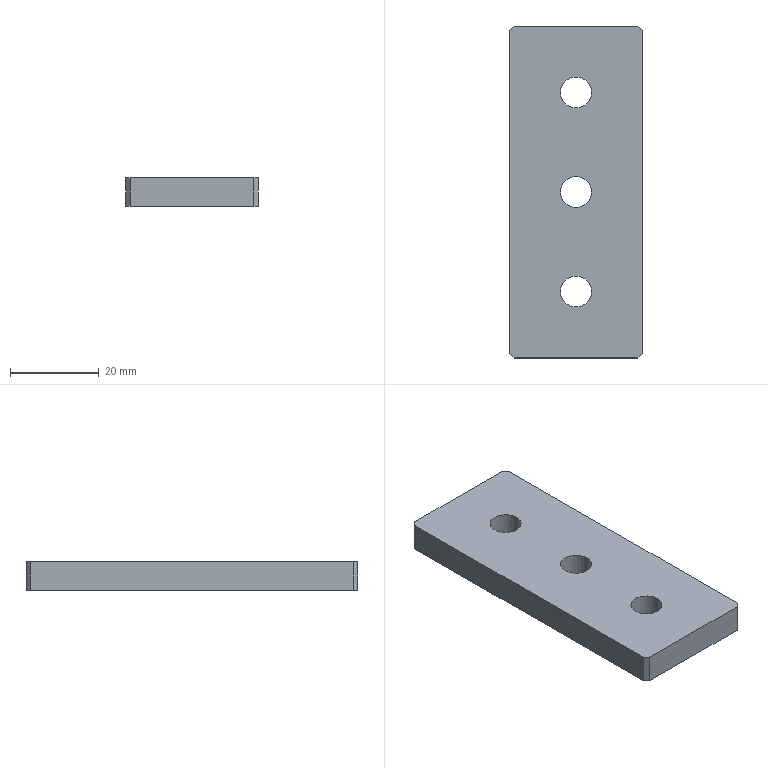Part | SolidWorks | features Chamfer 1, Extrusion 1, HoleWzd 1 | 1 solid | 16 faces | box 30 x 75 x 6.5 mm | volume 13862 mm3 | plane 10 | cylinder 6 | commonest cylinder face diameters 7 x6
STEP:
#1=CARTESIAN_POINT('',(-3.5,0.,0.));
#2=VERTEX_POINT('',#1);
#3=CARTESIAN_POINT('',(3.5,0.,0.));
#4=VERTEX_POINT('',#3);
#5=CARTESIAN_POINT('',(0.,0.,0.));
#6=DIRECTION('',(0.,0.,1.));
#7=DIRECTION('',(1.,0.,0.));
#8=AXIS2_PLACEMENT_3D('',#5,#6,#7);
#9=CIRCLE('',#8,3.5);
#10=EDGE_CURVE('',#2,#4,#9,.T.);
#11=ORIENTED_EDGE('',*,*,#10,.F.);
#12=CARTESIAN_POINT('',(-3.5,0.,6.5));
#13=VERTEX_POINT('',#12);
#14=CARTESIAN_POINT('',(-3.5,0.,6.5));
#15=DIRECTION('',(0.,0.,1.));
#16=VECTOR('',#15,1000.);
#17=LINE('',#14,#16);
#18=EDGE_CURVE('',#2,#13,#17,.T.);
#19=ORIENTED_EDGE('',*,*,#18,.T.);
#20=CARTESIAN_POINT('',(3.5,0.,6.5));
#21=VERTEX_POINT('',#20);
#22=CARTESIAN_POINT('',(0.,0.,6.5));
#23=DIRECTION('',(0.,0.,1.));
#24=DIRECTION('',(1.,0.,0.));
#25=AXIS2_PLACEMENT_3D('',#22,#23,#24);
#26=CIRCLE('',#25,3.5);
#27=EDGE_CURVE('',#13,#21,#26,.T.);
#28=ORIENTED_EDGE('',*,*,#27,.T.);
#29=CARTESIAN_POINT('',(3.5,0.,6.5));
#30=DIRECTION('',(0.,0.,1.));
#31=VECTOR('',#30,1000.);
#32=LINE('',#29,#31);
#33=EDGE_CURVE('',#4,#21,#32,.T.);
#34=ORIENTED_EDGE('',*,*,#33,.F.);
#35=EDGE_LOOP('',(#11,#19,#28,#34));
#36=FACE_OUTER_BOUND('',#35,.T.);
#37=CARTESIAN_POINT('',(0.,0.,6.5));
#38=DIRECTION('',(0.,0.,1.));
#39=DIRECTION('',(1.,0.,0.));
#40=AXIS2_PLACEMENT_3D('',#37,#38,#39);
#41=CYLINDRICAL_SURFACE('',#40,3.5);
#42=ADVANCED_FACE('',(#36),#41,.F.);
#43=CARTESIAN_POINT('',(-3.5,-22.5,0.));
#44=VERTEX_POINT('',#43);
#45=CARTESIAN_POINT('',(3.5,-22.5,0.));
#46=VERTEX_POINT('',#45);
#47=CARTESIAN_POINT('',(0.,-22.5,0.));
#48=DIRECTION('',(0.,0.,1.));
#49=DIRECTION('',(1.,0.,0.));
#50=AXIS2_PLACEMENT_3D('',#47,#48,#49);
#51=CIRCLE('',#50,3.5);
#52=EDGE_CURVE('',#44,#46,#51,.T.);
#53=ORIENTED_EDGE('',*,*,#52,.F.);
#54=CARTESIAN_POINT('',(-3.5,-22.5,6.5));
#55=VERTEX_POINT('',#54);
#56=CARTESIAN_POINT('',(-3.5,-22.5,6.5));
#57=DIRECTION('',(0.,0.,1.));
#58=VECTOR('',#57,1000.);
#59=LINE('',#56,#58);
#60=EDGE_CURVE('',#44,#55,#59,.T.);
#61=ORIENTED_EDGE('',*,*,#60,.T.);
#62=CARTESIAN_POINT('',(3.5,-22.5,6.5));
#63=VERTEX_POINT('',#62);
#64=CARTESIAN_POINT('',(0.,-22.5,6.5));
#65=DIRECTION('',(0.,0.,1.));
#66=DIRECTION('',(1.,0.,0.));
#67=AXIS2_PLACEMENT_3D('',#64,#65,#66);
#68=CIRCLE('',#67,3.5);
#69=EDGE_CURVE('',#55,#63,#68,.T.);
#70=ORIENTED_EDGE('',*,*,#69,.T.);
#71=CARTESIAN_POINT('',(3.5,-22.5,6.5));
#72=DIRECTION('',(0.,0.,1.));
#73=VECTOR('',#72,1000.);
#74=LINE('',#71,#73);
#75=EDGE_CURVE('',#46,#63,#74,.T.);
#76=ORIENTED_EDGE('',*,*,#75,.F.);
#77=EDGE_LOOP('',(#53,#61,#70,#76));
#78=FACE_OUTER_BOUND('',#77,.T.);
#79=CARTESIAN_POINT('',(0.,-22.5,6.5));
#80=DIRECTION('',(0.,0.,1.));
#81=DIRECTION('',(1.,0.,0.));
#82=AXIS2_PLACEMENT_3D('',#79,#80,#81);
#83=CYLINDRICAL_SURFACE('',#82,3.5);
#84=ADVANCED_FACE('',(#78),#83,.F.);
#85=CARTESIAN_POINT('',(-3.5,22.5,0.));
#86=VERTEX_POINT('',#85);
#87=CARTESIAN_POINT('',(3.5,22.5,0.));
#88=VERTEX_POINT('',#87);
#89=CARTESIAN_POINT('',(0.,22.5,0.));
#90=DIRECTION('',(0.,0.,1.));
#91=DIRECTION('',(1.,0.,0.));
#92=AXIS2_PLACEMENT_3D('',#89,#90,#91);
#93=CIRCLE('',#92,3.5);
#94=EDGE_CURVE('',#86,#88,#93,.T.);
#95=ORIENTED_EDGE('',*,*,#94,.F.);
#96=CARTESIAN_POINT('',(-3.5,22.5,6.5));
#97=VERTEX_POINT('',#96);
#98=CARTESIAN_POINT('',(-3.5,22.5,6.5));
#99=DIRECTION('',(0.,0.,1.));
#100=VECTOR('',#99,1000.);
#101=LINE('',#98,#100);
#102=EDGE_CURVE('',#86,#97,#101,.T.);
#103=ORIENTED_EDGE('',*,*,#102,.T.);
#104=CARTESIAN_POINT('',(3.5,22.5,6.5));
#105=VERTEX_POINT('',#104);
#106=CARTESIAN_POINT('',(0.,22.5,6.5));
#107=DIRECTION('',(0.,0.,1.));
#108=DIRECTION('',(1.,0.,0.));
#109=AXIS2_PLACEMENT_3D('',#106,#107,#108);
#110=CIRCLE('',#109,3.5);
#111=EDGE_CURVE('',#97,#105,#110,.T.);
#112=ORIENTED_EDGE('',*,*,#111,.T.);
#113=CARTESIAN_POINT('',(3.5,22.5,6.5));
#114=DIRECTION('',(0.,0.,1.));
#115=VECTOR('',#114,1000.);
#116=LINE('',#113,#115);
#117=EDGE_CURVE('',#88,#105,#116,.T.);
#118=ORIENTED_EDGE('',*,*,#117,.F.);
#119=EDGE_LOOP('',(#95,#103,#112,#118));
#120=FACE_OUTER_BOUND('',#119,.T.);
#121=CARTESIAN_POINT('',(0.,22.5,6.5));
#122=DIRECTION('',(0.,0.,1.));
#123=DIRECTION('',(1.,0.,0.));
#124=AXIS2_PLACEMENT_3D('',#121,#122,#123);
#125=CYLINDRICAL_SURFACE('',#124,3.5);
#126=ADVANCED_FACE('',(#120),#125,.F.);
#127=CARTESIAN_POINT('',(15.,-36.5,0.));
#128=VERTEX_POINT('',#127);
#129=CARTESIAN_POINT('',(15.,36.5,0.));
#130=VERTEX_POINT('',#129);
#131=CARTESIAN_POINT('',(15.,37.5,0.));
#132=DIRECTION('',(0.,1.,0.));
#133=VECTOR('',#132,1000.);
#134=LINE('',#131,#133);
#135=EDGE_CURVE('',#128,#130,#134,.T.);
#136=ORIENTED_EDGE('',*,*,#135,.T.);
#137=CARTESIAN_POINT('',(15.,36.5,6.5));
#138=VERTEX_POINT('',#137);
#139=CARTESIAN_POINT('',(15.,36.5,6.5));
#140=DIRECTION('',(0.,0.,1.));
#141=VECTOR('',#140,1000.);
#142=LINE('',#139,#141);
#143=EDGE_CURVE('',#130,#138,#142,.T.);
#144=ORIENTED_EDGE('',*,*,#143,.T.);
#145=CARTESIAN_POINT('',(15.,-36.5,6.5));
#146=VERTEX_POINT('',#145);
#147=CARTESIAN_POINT('',(15.,37.5,6.5));
#148=DIRECTION('',(0.,1.,0.));
#149=VECTOR('',#148,1000.);
#150=LINE('',#147,#149);
#151=EDGE_CURVE('',#146,#138,#150,.T.);
#152=ORIENTED_EDGE('',*,*,#151,.F.);
#153=CARTESIAN_POINT('',(15.,-36.5,6.5));
#154=DIRECTION('',(0.,0.,-1.));
#155=VECTOR('',#154,1000.);
#156=LINE('',#153,#155);
#157=EDGE_CURVE('',#146,#128,#156,.T.);
#158=ORIENTED_EDGE('',*,*,#157,.T.);
#159=EDGE_LOOP('',(#136,#144,#152,#158));
#160=FACE_OUTER_BOUND('',#159,.T.);
#161=CARTESIAN_POINT('',(15.,37.5,6.5));
#162=DIRECTION('',(-1.,0.,0.));
#163=DIRECTION('',(0.,-1.,0.));
#164=AXIS2_PLACEMENT_3D('',#161,#162,#163);
#165=PLANE('',#164);
#166=ADVANCED_FACE('',(#160),#165,.F.);
#167=CARTESIAN_POINT('',(14.,37.5,0.));
#168=VERTEX_POINT('',#167);
#169=CARTESIAN_POINT('',(-14.,37.5,0.));
#170=VERTEX_POINT('',#169);
#171=CARTESIAN_POINT('',(-15.,37.5,0.));
#172=DIRECTION('',(-1.,0.,0.));
#173=VECTOR('',#172,1000.);
#174=LINE('',#171,#173);
#175=EDGE_CURVE('',#168,#170,#174,.T.);
#176=ORIENTED_EDGE('',*,*,#175,.T.);
#177=CARTESIAN_POINT('',(-14.,37.5,6.5));
#178=VERTEX_POINT('',#177);
#179=CARTESIAN_POINT('',(-14.,37.5,6.5));
#180=DIRECTION('',(0.,0.,1.));
#181=VECTOR('',#180,1000.);
#182=LINE('',#179,#181);
#183=EDGE_CURVE('',#170,#178,#182,.T.);
#184=ORIENTED_EDGE('',*,*,#183,.T.);
#185=CARTESIAN_POINT('',(14.,37.5,6.5));
#186=VERTEX_POINT('',#185);
#187=CARTESIAN_POINT('',(-15.,37.5,6.5));
#188=DIRECTION('',(-1.,0.,0.));
#189=VECTOR('',#188,1000.);
#190=LINE('',#187,#189);
#191=EDGE_CURVE('',#186,#178,#190,.T.);
#192=ORIENTED_EDGE('',*,*,#191,.F.);
#193=CARTESIAN_POINT('',(14.,37.5,6.5));
#194=DIRECTION('',(0.,0.,-1.));
#195=VECTOR('',#194,1000.);
#196=LINE('',#193,#195);
#197=EDGE_CURVE('',#186,#168,#196,.T.);
#198=ORIENTED_EDGE('',*,*,#197,.T.);
#199=EDGE_LOOP('',(#176,#184,#192,#198));
#200=FACE_OUTER_BOUND('',#199,.T.);
#201=CARTESIAN_POINT('',(-15.,37.5,6.5));
#202=DIRECTION('',(0.,-1.,0.));
#203=DIRECTION('',(0.,0.,-1.));
#204=AXIS2_PLACEMENT_3D('',#201,#202,#203);
#205=PLANE('',#204);
#206=ADVANCED_FACE('',(#200),#205,.F.);
#207=CARTESIAN_POINT('',(-15.,36.5,6.5));
#208=VERTEX_POINT('',#207);
#209=CARTESIAN_POINT('',(-15.,-36.5,6.5));
#210=VERTEX_POINT('',#209);
#211=CARTESIAN_POINT('',(-15.,37.5,6.5));
#212=DIRECTION('',(0.,-1.,0.));
#213=VECTOR('',#212,1000.);
#214=LINE('',#211,#213);
#215=EDGE_CURVE('',#208,#210,#214,.T.);
#216=ORIENTED_EDGE('',*,*,#215,.F.);
#217=CARTESIAN_POINT('',(-15.,36.5,0.));
#218=VERTEX_POINT('',#217);
#219=CARTESIAN_POINT('',(-15.,36.5,6.5));
#220=DIRECTION('',(0.,0.,-1.));
#221=VECTOR('',#220,1000.);
#222=LINE('',#219,#221);
#223=EDGE_CURVE('',#208,#218,#222,.T.);
#224=ORIENTED_EDGE('',*,*,#223,.T.);
#225=CARTESIAN_POINT('',(-15.,-36.5,0.));
#226=VERTEX_POINT('',#225);
#227=CARTESIAN_POINT('',(-15.,37.5,0.));
#228=DIRECTION('',(0.,-1.,0.));
#229=VECTOR('',#228,1000.);
#230=LINE('',#227,#229);
#231=EDGE_CURVE('',#218,#226,#230,.T.);
#232=ORIENTED_EDGE('',*,*,#231,.T.);
#233=CARTESIAN_POINT('',(-15.,-36.5,6.5));
#234=DIRECTION('',(0.,0.,1.));
#235=VECTOR('',#234,1000.);
#236=LINE('',#233,#235);
#237=EDGE_CURVE('',#226,#210,#236,.T.);
#238=ORIENTED_EDGE('',*,*,#237,.T.);
#239=EDGE_LOOP('',(#216,#224,#232,#238));
#240=FACE_OUTER_BOUND('',#239,.T.);
#241=CARTESIAN_POINT('',(-15.,37.5,6.5));
#242=DIRECTION('',(1.,0.,0.));
#243=DIRECTION('',(0.,1.,0.));
#244=AXIS2_PLACEMENT_3D('',#241,#242,#243);
#245=PLANE('',#244);
#246=ADVANCED_FACE('',(#240),#245,.F.);
#247=CARTESIAN_POINT('',(-14.,-37.5,0.));
#248=VERTEX_POINT('',#247);
#249=CARTESIAN_POINT('',(14.,-37.5,0.));
#250=VERTEX_POINT('',#249);
#251=CARTESIAN_POINT('',(-15.,-37.5,0.));
#252=DIRECTION('',(1.,0.,0.));
#253=VECTOR('',#252,1000.);
#254=LINE('',#251,#253);
#255=EDGE_CURVE('',#248,#250,#254,.T.);
#256=ORIENTED_EDGE('',*,*,#255,.T.);
#257=CARTESIAN_POINT('',(14.,-37.5,6.5));
#258=VERTEX_POINT('',#257);
#259=CARTESIAN_POINT('',(14.,-37.5,6.5));
#260=DIRECTION('',(0.,0.,1.));
#261=VECTOR('',#260,1000.);
#262=LINE('',#259,#261);
#263=EDGE_CURVE('',#250,#258,#262,.T.);
#264=ORIENTED_EDGE('',*,*,#263,.T.);
#265=CARTESIAN_POINT('',(-14.,-37.5,6.5));
#266=VERTEX_POINT('',#265);
#267=CARTESIAN_POINT('',(-15.,-37.5,6.5));
#268=DIRECTION('',(1.,0.,0.));
#269=VECTOR('',#268,1000.);
#270=LINE('',#267,#269);
#271=EDGE_CURVE('',#266,#258,#270,.T.);
#272=ORIENTED_EDGE('',*,*,#271,.F.);
#273=CARTESIAN_POINT('',(-14.,-37.5,6.5));
#274=DIRECTION('',(0.,0.,-1.));
#275=VECTOR('',#274,1000.);
#276=LINE('',#273,#275);
#277=EDGE_CURVE('',#266,#248,#276,.T.);
#278=ORIENTED_EDGE('',*,*,#277,.T.);
#279=EDGE_LOOP('',(#256,#264,#272,#278));
#280=FACE_OUTER_BOUND('',#279,.T.);
#281=CARTESIAN_POINT('',(-15.,-37.5,6.5));
#282=DIRECTION('',(0.,1.,0.));
#283=DIRECTION('',(0.,0.,1.));
#284=AXIS2_PLACEMENT_3D('',#281,#282,#283);
#285=PLANE('',#284);
#286=ADVANCED_FACE('',(#280),#285,.F.);
#287=CARTESIAN_POINT('',(0.,0.,6.5));
#288=DIRECTION('',(0.,0.,1.));
#289=DIRECTION('',(1.,0.,0.));
#290=AXIS2_PLACEMENT_3D('',#287,#288,#289);
#291=CIRCLE('',#290,3.5);
#292=EDGE_CURVE('',#21,#13,#291,.T.);
#293=ORIENTED_EDGE('',*,*,#292,.F.);
#294=ORIENTED_EDGE('',*,*,#27,.F.);
#295=EDGE_LOOP('',(#293,#294));
#296=FACE_BOUND('',#295,.T.);
#297=CARTESIAN_POINT('',(0.,-22.5,6.5));
#298=DIRECTION('',(0.,0.,1.));
#299=DIRECTION('',(1.,0.,0.));
#300=AXIS2_PLACEMENT_3D('',#297,#298,#299);
#301=CIRCLE('',#300,3.5);
#302=EDGE_CURVE('',#63,#55,#301,.T.);
#303=ORIENTED_EDGE('',*,*,#302,.F.);
#304=ORIENTED_EDGE('',*,*,#69,.F.);
#305=EDGE_LOOP('',(#303,#304));
#306=FACE_BOUND('',#305,.T.);
#307=CARTESIAN_POINT('',(0.,22.5,6.5));
#308=DIRECTION('',(0.,0.,1.));
#309=DIRECTION('',(1.,0.,0.));
#310=AXIS2_PLACEMENT_3D('',#307,#308,#309);
#311=CIRCLE('',#310,3.5);
#312=EDGE_CURVE('',#105,#97,#311,.T.);
#313=ORIENTED_EDGE('',*,*,#312,.F.);
#314=ORIENTED_EDGE('',*,*,#111,.F.);
#315=EDGE_LOOP('',(#313,#314));
#316=FACE_BOUND('',#315,.T.);
#317=ORIENTED_EDGE('',*,*,#191,.T.);
#318=CARTESIAN_POINT('',(-25.75,25.75,6.5));
#319=DIRECTION('',(-0.7071,-0.7071,0.));
#320=VECTOR('',#319,1000.);
#321=LINE('',#318,#320);
#322=EDGE_CURVE('',#178,#208,#321,.T.);
#323=ORIENTED_EDGE('',*,*,#322,.T.);
#324=ORIENTED_EDGE('',*,*,#215,.T.);
#325=CARTESIAN_POINT('',(-25.75,-25.75,6.5));
#326=DIRECTION('',(0.7071,-0.7071,0.));
#327=VECTOR('',#326,1000.);
#328=LINE('',#325,#327);
#329=EDGE_CURVE('',#210,#266,#328,.T.);
#330=ORIENTED_EDGE('',*,*,#329,.T.);
#331=ORIENTED_EDGE('',*,*,#271,.T.);
#332=CARTESIAN_POINT('',(25.75,-25.75,6.5));
#333=DIRECTION('',(0.7071,0.7071,0.));
#334=VECTOR('',#333,1000.);
#335=LINE('',#332,#334);
#336=EDGE_CURVE('',#258,#146,#335,.T.);
#337=ORIENTED_EDGE('',*,*,#336,.T.);
#338=ORIENTED_EDGE('',*,*,#151,.T.);
#339=CARTESIAN_POINT('',(25.75,25.75,6.5));
#340=DIRECTION('',(-0.7071,0.7071,0.));
#341=VECTOR('',#340,1000.);
#342=LINE('',#339,#341);
#343=EDGE_CURVE('',#138,#186,#342,.T.);
#344=ORIENTED_EDGE('',*,*,#343,.T.);
#345=EDGE_LOOP('',(#317,#323,#324,#330,#331,#337,#338,#344));
#346=FACE_OUTER_BOUND('',#345,.T.);
#347=CARTESIAN_POINT('',(0.,0.,6.5));
#348=DIRECTION('',(0.,0.,1.));
#349=DIRECTION('',(1.,0.,0.));
#350=AXIS2_PLACEMENT_3D('',#347,#348,#349);
#351=PLANE('',#350);
#352=ADVANCED_FACE('',(#296,#306,#316,#346),#351,.T.);
#353=CARTESIAN_POINT('',(0.,0.,0.));
#354=DIRECTION('',(0.,0.,1.));
#355=DIRECTION('',(1.,0.,0.));
#356=AXIS2_PLACEMENT_3D('',#353,#354,#355);
#357=CIRCLE('',#356,3.5);
#358=EDGE_CURVE('',#4,#2,#357,.T.);
#359=ORIENTED_EDGE('',*,*,#358,.T.);
#360=ORIENTED_EDGE('',*,*,#10,.T.);
#361=EDGE_LOOP('',(#359,#360));
#362=FACE_BOUND('',#361,.T.);
#363=CARTESIAN_POINT('',(0.,-22.5,0.));
#364=DIRECTION('',(0.,0.,1.));
#365=DIRECTION('',(1.,0.,0.));
#366=AXIS2_PLACEMENT_3D('',#363,#364,#365);
#367=CIRCLE('',#366,3.5);
#368=EDGE_CURVE('',#46,#44,#367,.T.);
#369=ORIENTED_EDGE('',*,*,#368,.T.);
#370=ORIENTED_EDGE('',*,*,#52,.T.);
#371=EDGE_LOOP('',(#369,#370));
#372=FACE_BOUND('',#371,.T.);
#373=CARTESIAN_POINT('',(0.,22.5,0.));
#374=DIRECTION('',(0.,0.,1.));
#375=DIRECTION('',(1.,0.,0.));
#376=AXIS2_PLACEMENT_3D('',#373,#374,#375);
#377=CIRCLE('',#376,3.5);
#378=EDGE_CURVE('',#88,#86,#377,.T.);
#379=ORIENTED_EDGE('',*,*,#378,.T.);
#380=ORIENTED_EDGE('',*,*,#94,.T.);
#381=EDGE_LOOP('',(#379,#380));
#382=FACE_BOUND('',#381,.T.);
#383=ORIENTED_EDGE('',*,*,#231,.F.);
#384=CARTESIAN_POINT('',(-15.,36.5,0.));
#385=DIRECTION('',(0.7071,0.7071,0.));
#386=VECTOR('',#385,1000.);
#387=LINE('',#384,#386);
#388=EDGE_CURVE('',#218,#170,#387,.T.);
#389=ORIENTED_EDGE('',*,*,#388,.T.);
#390=ORIENTED_EDGE('',*,*,#175,.F.);
#391=CARTESIAN_POINT('',(14.,37.5,0.));
#392=DIRECTION('',(0.7071,-0.7071,0.));
#393=VECTOR('',#392,1000.);
#394=LINE('',#391,#393);
#395=EDGE_CURVE('',#168,#130,#394,.T.);
#396=ORIENTED_EDGE('',*,*,#395,.T.);
#397=ORIENTED_EDGE('',*,*,#135,.F.);
#398=CARTESIAN_POINT('',(15.,-36.5,0.));
#399=DIRECTION('',(-0.7071,-0.7071,0.));
#400=VECTOR('',#399,1000.);
#401=LINE('',#398,#400);
#402=EDGE_CURVE('',#128,#250,#401,.T.);
#403=ORIENTED_EDGE('',*,*,#402,.T.);
#404=ORIENTED_EDGE('',*,*,#255,.F.);
#405=CARTESIAN_POINT('',(-14.,-37.5,0.));
#406=DIRECTION('',(-0.7071,0.7071,0.));
#407=VECTOR('',#406,1000.);
#408=LINE('',#405,#407);
#409=EDGE_CURVE('',#248,#226,#408,.T.);
#410=ORIENTED_EDGE('',*,*,#409,.T.);
#411=EDGE_LOOP('',(#383,#389,#390,#396,#397,#403,#404,#410));
#412=FACE_OUTER_BOUND('',#411,.T.);
#413=CARTESIAN_POINT('',(0.,0.,0.));
#414=DIRECTION('',(0.,0.,1.));
#415=DIRECTION('',(1.,0.,0.));
#416=AXIS2_PLACEMENT_3D('',#413,#414,#415);
#417=PLANE('',#416);
#418=ADVANCED_FACE('',(#362,#372,#382,#412),#417,.F.);
#419=ORIENTED_EDGE('',*,*,#102,.F.);
#420=ORIENTED_EDGE('',*,*,#378,.F.);
#421=ORIENTED_EDGE('',*,*,#117,.T.);
#422=ORIENTED_EDGE('',*,*,#312,.T.);
#423=EDGE_LOOP('',(#419,#420,#421,#422));
#424=FACE_OUTER_BOUND('',#423,.T.);
#425=CARTESIAN_POINT('',(0.,22.5,6.5));
#426=DIRECTION('',(0.,0.,1.));
#427=DIRECTION('',(1.,0.,0.));
#428=AXIS2_PLACEMENT_3D('',#425,#426,#427);
#429=CYLINDRICAL_SURFACE('',#428,3.5);
#430=ADVANCED_FACE('',(#424),#429,.F.);
#431=ORIENTED_EDGE('',*,*,#60,.F.);
#432=ORIENTED_EDGE('',*,*,#368,.F.);
#433=ORIENTED_EDGE('',*,*,#75,.T.);
#434=ORIENTED_EDGE('',*,*,#302,.T.);
#435=EDGE_LOOP('',(#431,#432,#433,#434));
#436=FACE_OUTER_BOUND('',#435,.T.);
#437=CARTESIAN_POINT('',(0.,-22.5,6.5));
#438=DIRECTION('',(0.,0.,1.));
#439=DIRECTION('',(1.,0.,0.));
#440=AXIS2_PLACEMENT_3D('',#437,#438,#439);
#441=CYLINDRICAL_SURFACE('',#440,3.5);
#442=ADVANCED_FACE('',(#436),#441,.F.);
#443=ORIENTED_EDGE('',*,*,#18,.F.);
#444=ORIENTED_EDGE('',*,*,#358,.F.);
#445=ORIENTED_EDGE('',*,*,#33,.T.);
#446=ORIENTED_EDGE('',*,*,#292,.T.);
#447=EDGE_LOOP('',(#443,#444,#445,#446));
#448=FACE_OUTER_BOUND('',#447,.T.);
#449=CARTESIAN_POINT('',(0.,0.,6.5));
#450=DIRECTION('',(0.,0.,1.));
#451=DIRECTION('',(1.,0.,0.));
#452=AXIS2_PLACEMENT_3D('',#449,#450,#451);
#453=CYLINDRICAL_SURFACE('',#452,3.5);
#454=ADVANCED_FACE('',(#448),#453,.F.);
#455=ORIENTED_EDGE('',*,*,#322,.F.);
#456=ORIENTED_EDGE('',*,*,#183,.F.);
#457=ORIENTED_EDGE('',*,*,#388,.F.);
#458=ORIENTED_EDGE('',*,*,#223,.F.);
#459=EDGE_LOOP('',(#455,#456,#457,#458));
#460=FACE_OUTER_BOUND('',#459,.T.);
#461=CARTESIAN_POINT('',(-15.,36.5,6.5));
#462=DIRECTION('',(0.7071,-0.7071,0.));
#463=DIRECTION('',(0.,0.,-1.));
#464=AXIS2_PLACEMENT_3D('',#461,#462,#463);
#465=PLANE('',#464);
#466=ADVANCED_FACE('',(#460),#465,.F.);
#467=ORIENTED_EDGE('',*,*,#343,.F.);
#468=ORIENTED_EDGE('',*,*,#143,.F.);
#469=ORIENTED_EDGE('',*,*,#395,.F.);
#470=ORIENTED_EDGE('',*,*,#197,.F.);
#471=EDGE_LOOP('',(#467,#468,#469,#470));
#472=FACE_OUTER_BOUND('',#471,.T.);
#473=CARTESIAN_POINT('',(14.,37.5,6.5));
#474=DIRECTION('',(-0.7071,-0.7071,0.));
#475=DIRECTION('',(0.,0.,-1.));
#476=AXIS2_PLACEMENT_3D('',#473,#474,#475);
#477=PLANE('',#476);
#478=ADVANCED_FACE('',(#472),#477,.F.);
#479=ORIENTED_EDGE('',*,*,#336,.F.);
#480=ORIENTED_EDGE('',*,*,#263,.F.);
#481=ORIENTED_EDGE('',*,*,#402,.F.);
#482=ORIENTED_EDGE('',*,*,#157,.F.);
#483=EDGE_LOOP('',(#479,#480,#481,#482));
#484=FACE_OUTER_BOUND('',#483,.T.);
#485=CARTESIAN_POINT('',(15.,-36.5,6.5));
#486=DIRECTION('',(-0.7071,0.7071,0.));
#487=DIRECTION('',(0.,0.,-1.));
#488=AXIS2_PLACEMENT_3D('',#485,#486,#487);
#489=PLANE('',#488);
#490=ADVANCED_FACE('',(#484),#489,.F.);
#491=ORIENTED_EDGE('',*,*,#329,.F.);
#492=ORIENTED_EDGE('',*,*,#237,.F.);
#493=ORIENTED_EDGE('',*,*,#409,.F.);
#494=ORIENTED_EDGE('',*,*,#277,.F.);
#495=EDGE_LOOP('',(#491,#492,#493,#494));
#496=FACE_OUTER_BOUND('',#495,.T.);
#497=CARTESIAN_POINT('',(-14.,-37.5,6.5));
#498=DIRECTION('',(0.7071,0.7071,0.));
#499=DIRECTION('',(0.,0.,-1.));
#500=AXIS2_PLACEMENT_3D('',#497,#498,#499);
#501=PLANE('',#500);
#502=ADVANCED_FACE('',(#496),#501,.F.);
#503=CLOSED_SHELL('',(#42,#84,#126,#166,#206,#246,#286,#352,#418,#430,#442,#454,#466,#478,#490,#502));
#504=MANIFOLD_SOLID_BREP('',#503);
#505=CARTESIAN_POINT('',(0.,0.,0.));
#506=DIRECTION('',(0.,0.,1.));
#507=DIRECTION('',(1.,0.,0.));
#508=AXIS2_PLACEMENT_3D('',#505,#506,#507);
#509=(LENGTH_UNIT()NAMED_UNIT(*)SI_UNIT(.MILLI.,.METRE.));
#510=UNCERTAINTY_MEASURE_WITH_UNIT(LENGTH_MEASURE(0.00001),#509,'','');
#511=(NAMED_UNIT(*)PLANE_ANGLE_UNIT()SI_UNIT($,.RADIAN.));
#512=(NAMED_UNIT(*)SI_UNIT($,.STERADIAN.)SOLID_ANGLE_UNIT());
#513=(GEOMETRIC_REPRESENTATION_CONTEXT(3)GLOBAL_UNCERTAINTY_ASSIGNED_CONTEXT((#510))GLOBAL_UNIT_ASSIGNED_CONTEXT((#509,#511,#512))REPRESENTATION_CONTEXT('',''));
#514=ADVANCED_BREP_SHAPE_REPRESENTATION('',(#504,#508),#513);